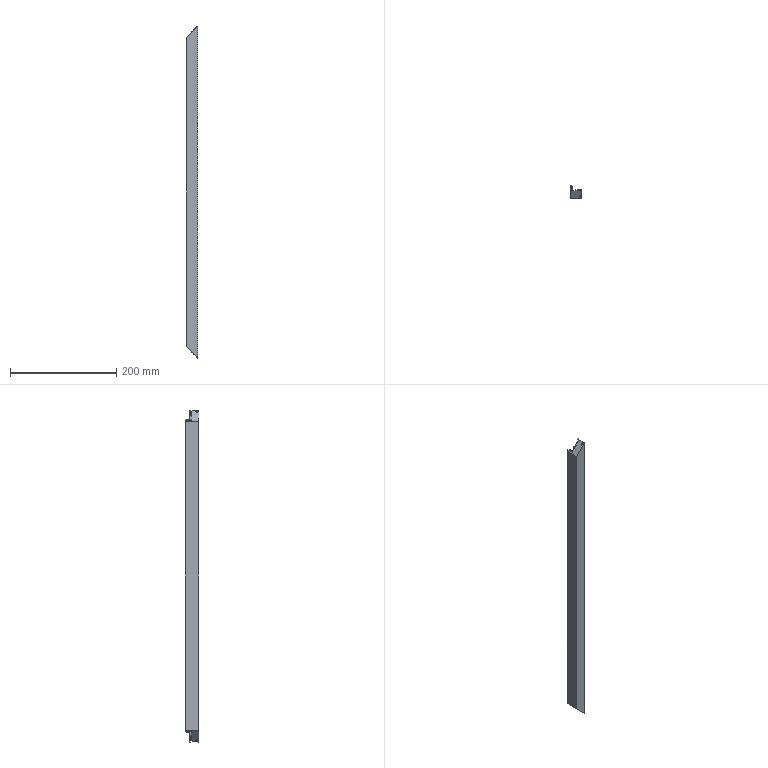Part | SolidWorks | features Extrusion 1, ICE 1 | 1 solid | 39 faces | box 22 x 25 x 624 mm | volume 198799 mm3 | plane 22 | cylinder 17 | commonest cylinder face diameters 0.6 x2 2 x2 3.8 x2 23.6 x2 26 x2 0.97 x1
STEP:
#1=CARTESIAN_POINT('',(27.064,65.097,604.634));
#2=VERTEX_POINT('',#1);
#3=CARTESIAN_POINT('',(26.938,66.899,604.509));
#4=VERTEX_POINT('',#3);
#5=CARTESIAN_POINT('',(27.064,65.097,604.634));
#6=CARTESIAN_POINT('',(26.98,65.694,604.55));
#7=CARTESIAN_POINT('',(26.938,66.296,604.509));
#8=CARTESIAN_POINT('',(26.938,66.899,604.509));
#9=(BOUNDED_CURVE()B_SPLINE_CURVE(3,(#5,#6,#7,#8),.UNSPECIFIED.,.F.,.F.)B_SPLINE_CURVE_WITH_KNOTS((4,4),(6.144,6.283),.UNSPECIFIED.)CURVE()GEOMETRIC_REPRESENTATION_ITEM()RATIONAL_B_SPLINE_CURVE((1.,0.9984,0.9984,1.))REPRESENTATION_ITEM(''));
#10=EDGE_CURVE('',#2,#4,#9,.T.);
#11=ORIENTED_EDGE('',*,*,#10,.T.);
#12=CARTESIAN_POINT('',(26.938,66.899,19.491));
#13=VERTEX_POINT('',#12);
#14=CARTESIAN_POINT('',(26.938,66.899,624.));
#15=DIRECTION('',(0.,0.,-1.));
#16=VECTOR('',#15,1000.);
#17=LINE('',#14,#16);
#18=EDGE_CURVE('',#4,#13,#17,.T.);
#19=ORIENTED_EDGE('',*,*,#18,.T.);
#20=CARTESIAN_POINT('',(27.064,65.097,19.366));
#21=VERTEX_POINT('',#20);
#22=CARTESIAN_POINT('',(26.938,66.899,19.491));
#23=CARTESIAN_POINT('',(26.938,66.296,19.491));
#24=CARTESIAN_POINT('',(26.98,65.694,19.45));
#25=CARTESIAN_POINT('',(27.064,65.097,19.366));
#26=(BOUNDED_CURVE()B_SPLINE_CURVE(3,(#22,#23,#24,#25),.UNSPECIFIED.,.F.,.F.)B_SPLINE_CURVE_WITH_KNOTS((4,4),(3.142,3.281),.UNSPECIFIED.)CURVE()GEOMETRIC_REPRESENTATION_ITEM()RATIONAL_B_SPLINE_CURVE((1.,0.9984,0.9984,1.))REPRESENTATION_ITEM(''));
#27=EDGE_CURVE('',#13,#21,#26,.T.);
#28=ORIENTED_EDGE('',*,*,#27,.T.);
#29=CARTESIAN_POINT('',(27.064,65.097,624.));
#30=DIRECTION('',(0.,0.,-1.));
#31=VECTOR('',#30,1000.);
#32=LINE('',#29,#31);
#33=EDGE_CURVE('',#2,#21,#32,.T.);
#34=ORIENTED_EDGE('',*,*,#33,.F.);
#35=EDGE_LOOP('',(#11,#19,#28,#34));
#36=FACE_OUTER_BOUND('',#35,.T.);
#37=CARTESIAN_POINT('',(39.938,66.899,624.));
#38=DIRECTION('',(0.,0.,-1.));
#39=DIRECTION('',(-1.,0.,0.));
#40=AXIS2_PLACEMENT_3D('',#37,#38,#39);
#41=CYLINDRICAL_SURFACE('',#40,13.);
#42=ADVANCED_FACE('',(#36),#41,.T.);
#43=CARTESIAN_POINT('',(28.252,68.536,605.823));
#44=VERTEX_POINT('',#43);
#45=CARTESIAN_POINT('',(28.138,66.899,605.709));
#46=VERTEX_POINT('',#45);
#47=CARTESIAN_POINT('',(28.252,68.536,605.823));
#48=CARTESIAN_POINT('',(28.176,67.993,605.747));
#49=CARTESIAN_POINT('',(28.138,67.447,605.709));
#50=CARTESIAN_POINT('',(28.138,66.899,605.709));
#51=(BOUNDED_CURVE()B_SPLINE_CURVE(3,(#47,#48,#49,#50),.UNSPECIFIED.,.F.,.F.)B_SPLINE_CURVE_WITH_KNOTS((4,4),(6.144,6.283),.UNSPECIFIED.)CURVE()GEOMETRIC_REPRESENTATION_ITEM()RATIONAL_B_SPLINE_CURVE((1.,0.9984,0.9984,1.))REPRESENTATION_ITEM(''));
#52=EDGE_CURVE('',#44,#46,#51,.T.);
#53=ORIENTED_EDGE('',*,*,#52,.T.);
#54=CARTESIAN_POINT('',(28.138,66.899,18.291));
#55=VERTEX_POINT('',#54);
#56=CARTESIAN_POINT('',(28.138,66.899,624.));
#57=DIRECTION('',(0.,0.,-1.));
#58=VECTOR('',#57,1000.);
#59=LINE('',#56,#58);
#60=EDGE_CURVE('',#46,#55,#59,.T.);
#61=ORIENTED_EDGE('',*,*,#60,.T.);
#62=CARTESIAN_POINT('',(28.252,68.536,18.177));
#63=VERTEX_POINT('',#62);
#64=CARTESIAN_POINT('',(28.138,66.899,18.291));
#65=CARTESIAN_POINT('',(28.138,67.447,18.291));
#66=CARTESIAN_POINT('',(28.176,67.993,18.253));
#67=CARTESIAN_POINT('',(28.252,68.536,18.177));
#68=(BOUNDED_CURVE()B_SPLINE_CURVE(3,(#64,#65,#66,#67),.UNSPECIFIED.,.F.,.F.)B_SPLINE_CURVE_WITH_KNOTS((4,4),(3.142,3.281),.UNSPECIFIED.)CURVE()GEOMETRIC_REPRESENTATION_ITEM()RATIONAL_B_SPLINE_CURVE((1.,0.9984,0.9984,1.))REPRESENTATION_ITEM(''));
#69=EDGE_CURVE('',#55,#63,#68,.T.);
#70=ORIENTED_EDGE('',*,*,#69,.T.);
#71=CARTESIAN_POINT('',(28.252,68.536,624.));
#72=DIRECTION('',(0.,0.,-1.));
#73=VECTOR('',#72,1000.);
#74=LINE('',#71,#73);
#75=EDGE_CURVE('',#44,#63,#74,.T.);
#76=ORIENTED_EDGE('',*,*,#75,.F.);
#77=EDGE_LOOP('',(#53,#61,#70,#76));
#78=FACE_OUTER_BOUND('',#77,.T.);
#79=CARTESIAN_POINT('',(39.938,66.899,624.));
#80=DIRECTION('',(0.,0.,-1.));
#81=DIRECTION('',(-1.,0.,0.));
#82=AXIS2_PLACEMENT_3D('',#79,#80,#81);
#83=CYLINDRICAL_SURFACE('',#82,11.8);
#84=ADVANCED_FACE('',(#78),#83,.F.);
#85=CARTESIAN_POINT('',(44.608,52.847,622.178));
#86=VERTEX_POINT('',#85);
#87=CARTESIAN_POINT('',(41.6,51.304,619.17));
#88=VERTEX_POINT('',#87);
#89=CARTESIAN_POINT('',(44.608,52.847,622.178));
#90=CARTESIAN_POINT('',(43.172,53.878,620.743));
#91=CARTESIAN_POINT('',(41.6,53.071,619.17));
#92=CARTESIAN_POINT('',(41.6,51.304,619.17));
#93=(BOUNDED_CURVE()B_SPLINE_CURVE(3,(#89,#90,#91,#92),.UNSPECIFIED.,.F.,.F.)B_SPLINE_CURVE_WITH_KNOTS((4,4),(4.09,6.283),.UNSPECIFIED.)CURVE()GEOMETRIC_REPRESENTATION_ITEM()RATIONAL_B_SPLINE_CURVE((1.,0.6376,0.6376,1.))REPRESENTATION_ITEM(''));
#94=EDGE_CURVE('',#86,#88,#93,.T.);
#95=ORIENTED_EDGE('',*,*,#94,.T.);
#96=CARTESIAN_POINT('',(41.6,51.304,4.83));
#97=VERTEX_POINT('',#96);
#98=CARTESIAN_POINT('',(41.6,51.304,624.));
#99=DIRECTION('',(0.,0.,-1.));
#100=VECTOR('',#99,1000.);
#101=LINE('',#98,#100);
#102=EDGE_CURVE('',#88,#97,#101,.T.);
#103=ORIENTED_EDGE('',*,*,#102,.T.);
#104=CARTESIAN_POINT('',(44.608,52.847,1.822));
#105=VERTEX_POINT('',#104);
#106=CARTESIAN_POINT('',(41.6,51.304,4.83));
#107=CARTESIAN_POINT('',(41.6,53.071,4.83));
#108=CARTESIAN_POINT('',(43.172,53.878,3.257));
#109=CARTESIAN_POINT('',(44.608,52.847,1.822));
#110=(BOUNDED_CURVE()B_SPLINE_CURVE(3,(#106,#107,#108,#109),.UNSPECIFIED.,.F.,.F.)B_SPLINE_CURVE_WITH_KNOTS((4,4),(3.142,5.335),.UNSPECIFIED.)CURVE()GEOMETRIC_REPRESENTATION_ITEM()RATIONAL_B_SPLINE_CURVE((1.,0.6376,0.6376,1.))REPRESENTATION_ITEM(''));
#111=EDGE_CURVE('',#97,#105,#110,.T.);
#112=ORIENTED_EDGE('',*,*,#111,.T.);
#113=CARTESIAN_POINT('',(44.608,52.847,624.));
#114=DIRECTION('',(0.,0.,-1.));
#115=VECTOR('',#114,1000.);
#116=LINE('',#113,#115);
#117=EDGE_CURVE('',#86,#105,#116,.T.);
#118=ORIENTED_EDGE('',*,*,#117,.F.);
#119=EDGE_LOOP('',(#95,#103,#112,#118));
#120=FACE_OUTER_BOUND('',#119,.T.);
#121=CARTESIAN_POINT('',(43.5,51.304,624.));
#122=DIRECTION('',(0.,0.,-1.));
#123=DIRECTION('',(-1.,0.,0.));
#124=AXIS2_PLACEMENT_3D('',#121,#122,#123);
#125=CYLINDRICAL_SURFACE('',#124,1.9);
#126=ADVANCED_FACE('',(#120),#125,.F.);
#127=CARTESIAN_POINT('',(45.44,49.348,623.01));
#128=VERTEX_POINT('',#127);
#129=CARTESIAN_POINT('',(45.43,49.204,623.));
#130=VERTEX_POINT('',#129);
#131=CARTESIAN_POINT('',(45.44,49.348,623.01));
#132=CARTESIAN_POINT('',(45.433,49.3,623.003));
#133=CARTESIAN_POINT('',(45.43,49.252,623.));
#134=CARTESIAN_POINT('',(45.43,49.204,623.));
#135=(BOUNDED_CURVE()B_SPLINE_CURVE(3,(#131,#132,#133,#134),.UNSPECIFIED.,.F.,.F.)B_SPLINE_CURVE_WITH_KNOTS((4,4),(6.138,6.283),.UNSPECIFIED.)CURVE()GEOMETRIC_REPRESENTATION_ITEM()RATIONAL_B_SPLINE_CURVE((1.,0.9983,0.9983,1.))REPRESENTATION_ITEM(''));
#136=EDGE_CURVE('',#128,#130,#135,.T.);
#137=ORIENTED_EDGE('',*,*,#136,.T.);
#138=CARTESIAN_POINT('',(45.43,49.204,1.));
#139=VERTEX_POINT('',#138);
#140=CARTESIAN_POINT('',(45.43,49.204,624.));
#141=DIRECTION('',(0.,0.,-1.));
#142=VECTOR('',#141,1000.);
#143=LINE('',#140,#142);
#144=EDGE_CURVE('',#130,#139,#143,.T.);
#145=ORIENTED_EDGE('',*,*,#144,.T.);
#146=CARTESIAN_POINT('',(45.44,49.348,0.9896));
#147=VERTEX_POINT('',#146);
#148=CARTESIAN_POINT('',(45.43,49.204,1.));
#149=CARTESIAN_POINT('',(45.43,49.252,1.));
#150=CARTESIAN_POINT('',(45.433,49.3,0.9965));
#151=CARTESIAN_POINT('',(45.44,49.348,0.9896));
#152=(BOUNDED_CURVE()B_SPLINE_CURVE(3,(#148,#149,#150,#151),.UNSPECIFIED.,.F.,.F.)B_SPLINE_CURVE_WITH_KNOTS((4,4),(3.142,3.286),.UNSPECIFIED.)CURVE()GEOMETRIC_REPRESENTATION_ITEM()RATIONAL_B_SPLINE_CURVE((1.,0.9983,0.9983,1.))REPRESENTATION_ITEM(''));
#153=EDGE_CURVE('',#139,#147,#152,.T.);
#154=ORIENTED_EDGE('',*,*,#153,.T.);
#155=CARTESIAN_POINT('',(45.44,49.348,624.));
#156=DIRECTION('',(0.,0.,-1.));
#157=VECTOR('',#156,1000.);
#158=LINE('',#155,#157);
#159=EDGE_CURVE('',#128,#147,#158,.T.);
#160=ORIENTED_EDGE('',*,*,#159,.F.);
#161=EDGE_LOOP('',(#137,#145,#154,#160));
#162=FACE_OUTER_BOUND('',#161,.T.);
#163=CARTESIAN_POINT('',(46.43,49.204,624.));
#164=DIRECTION('',(0.,0.,-1.));
#165=DIRECTION('',(-1.,0.,0.));
#166=AXIS2_PLACEMENT_3D('',#163,#164,#165);
#167=CYLINDRICAL_SURFACE('',#166,1.);
#168=ADVANCED_FACE('',(#162),#167,.F.);
#169=CARTESIAN_POINT('',(24.43,73.204,602.));
#170=VERTEX_POINT('',#169);
#171=CARTESIAN_POINT('',(24.43,73.204,22.));
#172=VERTEX_POINT('',#171);
#173=CARTESIAN_POINT('',(24.43,73.204,624.));
#174=DIRECTION('',(0.,0.,-1.));
#175=VECTOR('',#174,1000.);
#176=LINE('',#173,#175);
#177=EDGE_CURVE('',#170,#172,#176,.T.);
#178=ORIENTED_EDGE('',*,*,#177,.T.);
#179=CARTESIAN_POINT('',(24.43,48.204,22.));
#180=VERTEX_POINT('',#179);
#181=CARTESIAN_POINT('',(24.43,78.204,22.));
#182=DIRECTION('',(0.,-1.,0.));
#183=VECTOR('',#182,1000.);
#184=LINE('',#181,#183);
#185=EDGE_CURVE('',#172,#180,#184,.T.);
#186=ORIENTED_EDGE('',*,*,#185,.T.);
#187=CARTESIAN_POINT('',(24.43,48.204,602.));
#188=VERTEX_POINT('',#187);
#189=CARTESIAN_POINT('',(24.43,48.204,624.));
#190=DIRECTION('',(0.,0.,-1.));
#191=VECTOR('',#190,1000.);
#192=LINE('',#189,#191);
#193=EDGE_CURVE('',#188,#180,#192,.T.);
#194=ORIENTED_EDGE('',*,*,#193,.F.);
#195=CARTESIAN_POINT('',(24.43,78.204,602.));
#196=DIRECTION('',(0.,-1.,0.));
#197=VECTOR('',#196,1000.);
#198=LINE('',#195,#197);
#199=EDGE_CURVE('',#170,#188,#198,.T.);
#200=ORIENTED_EDGE('',*,*,#199,.F.);
#201=EDGE_LOOP('',(#178,#186,#194,#200));
#202=FACE_OUTER_BOUND('',#201,.T.);
#203=CARTESIAN_POINT('',(24.43,48.204,624.));
#204=DIRECTION('',(1.,0.,0.));
#205=DIRECTION('',(0.,0.,-1.));
#206=AXIS2_PLACEMENT_3D('',#203,#204,#205);
#207=PLANE('',#206);
#208=ADVANCED_FACE('',(#202),#207,.F.);
#209=ORIENTED_EDGE('',*,*,#193,.T.);
#210=CARTESIAN_POINT('',(46.43,48.204,0.));
#211=VERTEX_POINT('',#210);
#212=CARTESIAN_POINT('',(24.43,48.204,22.));
#213=DIRECTION('',(-0.7071,0.,0.7071));
#214=VECTOR('',#213,1000.);
#215=LINE('',#212,#214);
#216=EDGE_CURVE('',#211,#180,#215,.T.);
#217=ORIENTED_EDGE('',*,*,#216,.F.);
#218=CARTESIAN_POINT('',(46.43,48.204,624.));
#219=VERTEX_POINT('',#218);
#220=CARTESIAN_POINT('',(46.43,48.204,624.));
#221=DIRECTION('',(0.,0.,-1.));
#222=VECTOR('',#221,1000.);
#223=LINE('',#220,#222);
#224=EDGE_CURVE('',#219,#211,#223,.T.);
#225=ORIENTED_EDGE('',*,*,#224,.F.);
#226=CARTESIAN_POINT('',(24.43,48.204,602.));
#227=DIRECTION('',(0.7071,0.,0.7071));
#228=VECTOR('',#227,1000.);
#229=LINE('',#226,#228);
#230=EDGE_CURVE('',#188,#219,#229,.T.);
#231=ORIENTED_EDGE('',*,*,#230,.F.);
#232=EDGE_LOOP('',(#209,#217,#225,#231));
#233=FACE_OUTER_BOUND('',#232,.T.);
#234=CARTESIAN_POINT('',(24.43,48.204,624.));
#235=DIRECTION('',(0.,1.,0.));
#236=DIRECTION('',(0.,0.,1.));
#237=AXIS2_PLACEMENT_3D('',#234,#235,#236);
#238=PLANE('',#237);
#239=ADVANCED_FACE('',(#233),#238,.F.);
#240=ORIENTED_EDGE('',*,*,#144,.F.);
#241=CARTESIAN_POINT('',(45.43,49.204,623.));
#242=CARTESIAN_POINT('',(45.43,48.618,623.));
#243=CARTESIAN_POINT('',(45.844,48.204,623.414));
#244=CARTESIAN_POINT('',(46.43,48.204,624.));
#245=(BOUNDED_CURVE()B_SPLINE_CURVE(3,(#241,#242,#243,#244),.UNSPECIFIED.,.F.,.F.)B_SPLINE_CURVE_WITH_KNOTS((4,4),(0.,1.571),.UNSPECIFIED.)CURVE()GEOMETRIC_REPRESENTATION_ITEM()RATIONAL_B_SPLINE_CURVE((1.,0.8047,0.8047,1.))REPRESENTATION_ITEM(''));
#246=EDGE_CURVE('',#130,#219,#245,.T.);
#247=ORIENTED_EDGE('',*,*,#246,.T.);
#248=ORIENTED_EDGE('',*,*,#224,.T.);
#249=CARTESIAN_POINT('',(46.43,48.204,0.));
#250=CARTESIAN_POINT('',(45.844,48.204,0.5858));
#251=CARTESIAN_POINT('',(45.43,48.618,1.));
#252=CARTESIAN_POINT('',(45.43,49.204,1.));
#253=(BOUNDED_CURVE()B_SPLINE_CURVE(3,(#249,#250,#251,#252),.UNSPECIFIED.,.F.,.F.)B_SPLINE_CURVE_WITH_KNOTS((4,4),(1.571,3.142),.UNSPECIFIED.)CURVE()GEOMETRIC_REPRESENTATION_ITEM()RATIONAL_B_SPLINE_CURVE((1.,0.8047,0.8047,1.))REPRESENTATION_ITEM(''));
#254=EDGE_CURVE('',#211,#139,#253,.T.);
#255=ORIENTED_EDGE('',*,*,#254,.T.);
#256=EDGE_LOOP('',(#240,#247,#248,#255));
#257=FACE_OUTER_BOUND('',#256,.T.);
#258=CARTESIAN_POINT('',(46.43,49.204,624.));
#259=DIRECTION('',(0.,0.,-1.));
#260=DIRECTION('',(-1.,0.,0.));
#261=AXIS2_PLACEMENT_3D('',#258,#259,#260);
#262=CYLINDRICAL_SURFACE('',#261,1.);
#263=ADVANCED_FACE('',(#257),#262,.F.);
#264=ORIENTED_EDGE('',*,*,#159,.T.);
#265=CARTESIAN_POINT('',(44.663,49.801,1.767));
#266=VERTEX_POINT('',#265);
#267=CARTESIAN_POINT('',(45.44,49.348,0.9896));
#268=CARTESIAN_POINT('',(45.514,49.857,0.9153));
#269=CARTESIAN_POINT('',(45.07,50.116,1.36));
#270=CARTESIAN_POINT('',(44.663,49.801,1.767));
#271=(BOUNDED_CURVE()B_SPLINE_CURVE(3,(#267,#268,#269,#270),.UNSPECIFIED.,.F.,.F.)B_SPLINE_CURVE_WITH_KNOTS((4,4),(6.138,8.513),.UNSPECIFIED.)CURVE()GEOMETRIC_REPRESENTATION_ITEM()RATIONAL_B_SPLINE_CURVE((1.,0.5828,0.5828,1.))REPRESENTATION_ITEM(''));
#272=EDGE_CURVE('',#147,#266,#271,.T.);
#273=ORIENTED_EDGE('',*,*,#272,.T.);
#274=CARTESIAN_POINT('',(44.663,49.801,622.233));
#275=VERTEX_POINT('',#274);
#276=CARTESIAN_POINT('',(44.663,49.801,624.));
#277=DIRECTION('',(0.,0.,-1.));
#278=VECTOR('',#277,1000.);
#279=LINE('',#276,#278);
#280=EDGE_CURVE('',#275,#266,#279,.T.);
#281=ORIENTED_EDGE('',*,*,#280,.F.);
#282=CARTESIAN_POINT('',(44.663,49.801,622.233));
#283=CARTESIAN_POINT('',(45.07,50.116,622.64));
#284=CARTESIAN_POINT('',(45.514,49.857,623.085));
#285=CARTESIAN_POINT('',(45.44,49.348,623.01));
#286=(BOUNDED_CURVE()B_SPLINE_CURVE(3,(#282,#283,#284,#285),.UNSPECIFIED.,.F.,.F.)B_SPLINE_CURVE_WITH_KNOTS((4,4),(0.9119,3.286),.UNSPECIFIED.)CURVE()GEOMETRIC_REPRESENTATION_ITEM()RATIONAL_B_SPLINE_CURVE((1.,0.5828,0.5828,1.))REPRESENTATION_ITEM(''));
#287=EDGE_CURVE('',#275,#128,#286,.T.);
#288=ORIENTED_EDGE('',*,*,#287,.T.);
#289=EDGE_LOOP('',(#264,#273,#281,#288));
#290=FACE_OUTER_BOUND('',#289,.T.);
#291=CARTESIAN_POINT('',(44.96,49.418,624.));
#292=DIRECTION('',(0.,0.,-1.));
#293=DIRECTION('',(-1.,0.,0.));
#294=AXIS2_PLACEMENT_3D('',#291,#292,#293);
#295=CYLINDRICAL_SURFACE('',#294,0.4852);
#296=ADVANCED_FACE('',(#290),#295,.T.);
#297=ORIENTED_EDGE('',*,*,#102,.F.);
#298=CARTESIAN_POINT('',(41.6,51.304,619.17));
#299=CARTESIAN_POINT('',(41.6,49.489,619.17));
#300=CARTESIAN_POINT('',(43.228,48.691,620.799));
#301=CARTESIAN_POINT('',(44.663,49.801,622.233));
#302=(BOUNDED_CURVE()B_SPLINE_CURVE(3,(#298,#299,#300,#301),.UNSPECIFIED.,.F.,.F.)B_SPLINE_CURVE_WITH_KNOTS((4,4),(0.,2.23),.UNSPECIFIED.)CURVE()GEOMETRIC_REPRESENTATION_ITEM()RATIONAL_B_SPLINE_CURVE((1.,0.6269,0.6269,1.))REPRESENTATION_ITEM(''));
#303=EDGE_CURVE('',#88,#275,#302,.T.);
#304=ORIENTED_EDGE('',*,*,#303,.T.);
#305=ORIENTED_EDGE('',*,*,#280,.T.);
#306=CARTESIAN_POINT('',(44.663,49.801,1.767));
#307=CARTESIAN_POINT('',(43.228,48.691,3.201));
#308=CARTESIAN_POINT('',(41.6,49.489,4.83));
#309=CARTESIAN_POINT('',(41.6,51.304,4.83));
#310=(BOUNDED_CURVE()B_SPLINE_CURVE(3,(#306,#307,#308,#309),.UNSPECIFIED.,.F.,.F.)B_SPLINE_CURVE_WITH_KNOTS((4,4),(0.9119,3.142),.UNSPECIFIED.)CURVE()GEOMETRIC_REPRESENTATION_ITEM()RATIONAL_B_SPLINE_CURVE((1.,0.6269,0.6269,1.))REPRESENTATION_ITEM(''));
#311=EDGE_CURVE('',#266,#97,#310,.T.);
#312=ORIENTED_EDGE('',*,*,#311,.T.);
#313=EDGE_LOOP('',(#297,#304,#305,#312));
#314=FACE_OUTER_BOUND('',#313,.T.);
#315=CARTESIAN_POINT('',(43.5,51.304,624.));
#316=DIRECTION('',(0.,0.,-1.));
#317=DIRECTION('',(-1.,0.,0.));
#318=AXIS2_PLACEMENT_3D('',#315,#316,#317);
#319=CYLINDRICAL_SURFACE('',#318,1.9);
#320=ADVANCED_FACE('',(#314),#319,.F.);
#321=ORIENTED_EDGE('',*,*,#117,.T.);
#322=CARTESIAN_POINT('',(45.4,53.253,1.03));
#323=VERTEX_POINT('',#322);
#324=CARTESIAN_POINT('',(44.608,52.847,1.822));
#325=CARTESIAN_POINT('',(44.986,52.575,1.444));
#326=CARTESIAN_POINT('',(45.4,52.788,1.03));
#327=CARTESIAN_POINT('',(45.4,53.253,1.03));
#328=(BOUNDED_CURVE()B_SPLINE_CURVE(3,(#324,#325,#326,#327),.UNSPECIFIED.,.F.,.F.)B_SPLINE_CURVE_WITH_KNOTS((4,4),(4.09,6.283),.UNSPECIFIED.)CURVE()GEOMETRIC_REPRESENTATION_ITEM()RATIONAL_B_SPLINE_CURVE((1.,0.6376,0.6376,1.))REPRESENTATION_ITEM(''));
#329=EDGE_CURVE('',#105,#323,#328,.T.);
#330=ORIENTED_EDGE('',*,*,#329,.T.);
#331=CARTESIAN_POINT('',(45.4,53.253,622.97));
#332=VERTEX_POINT('',#331);
#333=CARTESIAN_POINT('',(45.4,53.253,624.));
#334=DIRECTION('',(0.,0.,-1.));
#335=VECTOR('',#334,1000.);
#336=LINE('',#333,#335);
#337=EDGE_CURVE('',#332,#323,#336,.T.);
#338=ORIENTED_EDGE('',*,*,#337,.F.);
#339=CARTESIAN_POINT('',(45.4,53.253,622.97));
#340=CARTESIAN_POINT('',(45.4,52.788,622.97));
#341=CARTESIAN_POINT('',(44.986,52.575,622.556));
#342=CARTESIAN_POINT('',(44.608,52.847,622.178));
#343=(BOUNDED_CURVE()B_SPLINE_CURVE(3,(#339,#340,#341,#342),.UNSPECIFIED.,.F.,.F.)B_SPLINE_CURVE_WITH_KNOTS((4,4),(3.142,5.335),.UNSPECIFIED.)CURVE()GEOMETRIC_REPRESENTATION_ITEM()RATIONAL_B_SPLINE_CURVE((1.,0.6376,0.6376,1.))REPRESENTATION_ITEM(''));
#344=EDGE_CURVE('',#332,#86,#343,.T.);
#345=ORIENTED_EDGE('',*,*,#344,.T.);
#346=EDGE_LOOP('',(#321,#330,#338,#345));
#347=FACE_OUTER_BOUND('',#346,.T.);
#348=CARTESIAN_POINT('',(44.9,53.253,624.));
#349=DIRECTION('',(0.,0.,-1.));
#350=DIRECTION('',(-1.,0.,0.));
#351=AXIS2_PLACEMENT_3D('',#348,#349,#350);
#352=CYLINDRICAL_SURFACE('',#351,0.5);
#353=ADVANCED_FACE('',(#347),#352,.T.);
#354=ORIENTED_EDGE('',*,*,#337,.T.);
#355=CARTESIAN_POINT('',(45.4,58.567,1.03));
#356=VERTEX_POINT('',#355);
#357=CARTESIAN_POINT('',(45.4,58.567,1.03));
#358=DIRECTION('',(0.,1.,0.));
#359=VECTOR('',#358,1000.);
#360=LINE('',#357,#359);
#361=EDGE_CURVE('',#323,#356,#360,.T.);
#362=ORIENTED_EDGE('',*,*,#361,.T.);
#363=CARTESIAN_POINT('',(45.4,58.567,622.97));
#364=VERTEX_POINT('',#363);
#365=CARTESIAN_POINT('',(45.4,58.567,624.));
#366=DIRECTION('',(0.,0.,-1.));
#367=VECTOR('',#366,1000.);
#368=LINE('',#365,#367);
#369=EDGE_CURVE('',#364,#356,#368,.T.);
#370=ORIENTED_EDGE('',*,*,#369,.F.);
#371=CARTESIAN_POINT('',(45.4,58.567,622.97));
#372=DIRECTION('',(0.,-1.,0.));
#373=VECTOR('',#372,1000.);
#374=LINE('',#371,#373);
#375=EDGE_CURVE('',#364,#332,#374,.T.);
#376=ORIENTED_EDGE('',*,*,#375,.T.);
#377=EDGE_LOOP('',(#354,#362,#370,#376));
#378=FACE_OUTER_BOUND('',#377,.T.);
#379=CARTESIAN_POINT('',(45.4,58.567,624.));
#380=DIRECTION('',(-1.,0.,0.));
#381=DIRECTION('',(0.,0.,1.));
#382=AXIS2_PLACEMENT_3D('',#379,#380,#381);
#383=PLANE('',#382);
#384=ADVANCED_FACE('',(#378),#383,.F.);
#385=ORIENTED_EDGE('',*,*,#369,.T.);
#386=CARTESIAN_POINT('',(41.4,62.567,5.03));
#387=VERTEX_POINT('',#386);
#388=CARTESIAN_POINT('',(45.4,58.567,1.03));
#389=CARTESIAN_POINT('',(45.4,60.91,1.03));
#390=CARTESIAN_POINT('',(43.743,62.567,2.687));
#391=CARTESIAN_POINT('',(41.4,62.567,5.03));
#392=(BOUNDED_CURVE()B_SPLINE_CURVE(3,(#388,#389,#390,#391),.UNSPECIFIED.,.F.,.F.)B_SPLINE_CURVE_WITH_KNOTS((4,4),(0.,1.571),.UNSPECIFIED.)CURVE()GEOMETRIC_REPRESENTATION_ITEM()RATIONAL_B_SPLINE_CURVE((1.,0.8047,0.8047,1.))REPRESENTATION_ITEM(''));
#393=EDGE_CURVE('',#356,#387,#392,.T.);
#394=ORIENTED_EDGE('',*,*,#393,.T.);
#395=CARTESIAN_POINT('',(41.4,62.567,618.97));
#396=VERTEX_POINT('',#395);
#397=CARTESIAN_POINT('',(41.4,62.567,624.));
#398=DIRECTION('',(0.,0.,-1.));
#399=VECTOR('',#398,1000.);
#400=LINE('',#397,#399);
#401=EDGE_CURVE('',#396,#387,#400,.T.);
#402=ORIENTED_EDGE('',*,*,#401,.F.);
#403=CARTESIAN_POINT('',(41.4,62.567,618.97));
#404=CARTESIAN_POINT('',(43.743,62.567,621.313));
#405=CARTESIAN_POINT('',(45.4,60.91,622.97));
#406=CARTESIAN_POINT('',(45.4,58.567,622.97));
#407=(BOUNDED_CURVE()B_SPLINE_CURVE(3,(#403,#404,#405,#406),.UNSPECIFIED.,.F.,.F.)B_SPLINE_CURVE_WITH_KNOTS((4,4),(1.571,3.142),.UNSPECIFIED.)CURVE()GEOMETRIC_REPRESENTATION_ITEM()RATIONAL_B_SPLINE_CURVE((1.,0.8047,0.8047,1.))REPRESENTATION_ITEM(''));
#408=EDGE_CURVE('',#396,#364,#407,.T.);
#409=ORIENTED_EDGE('',*,*,#408,.T.);
#410=EDGE_LOOP('',(#385,#394,#402,#409));
#411=FACE_OUTER_BOUND('',#410,.T.);
#412=CARTESIAN_POINT('',(41.4,58.567,624.));
#413=DIRECTION('',(0.,0.,-1.));
#414=DIRECTION('',(-1.,0.,0.));
#415=AXIS2_PLACEMENT_3D('',#412,#413,#414);
#416=CYLINDRICAL_SURFACE('',#415,4.);
#417=ADVANCED_FACE('',(#411),#416,.T.);
#418=ORIENTED_EDGE('',*,*,#401,.T.);
#419=CARTESIAN_POINT('',(35.32,62.567,11.11));
#420=VERTEX_POINT('',#419);
#421=CARTESIAN_POINT('',(-271.125,62.567,317.555));
#422=DIRECTION('',(-0.7071,0.,0.7071));
#423=VECTOR('',#422,1000.);
#424=LINE('',#421,#423);
#425=EDGE_CURVE('',#387,#420,#424,.T.);
#426=ORIENTED_EDGE('',*,*,#425,.T.);
#427=CARTESIAN_POINT('',(35.32,62.567,612.89));
#428=VERTEX_POINT('',#427);
#429=CARTESIAN_POINT('',(35.32,62.567,624.));
#430=DIRECTION('',(0.,0.,-1.));
#431=VECTOR('',#430,1000.);
#432=LINE('',#429,#431);
#433=EDGE_CURVE('',#428,#420,#432,.T.);
#434=ORIENTED_EDGE('',*,*,#433,.F.);
#435=CARTESIAN_POINT('',(40.875,62.567,618.445));
#436=DIRECTION('',(0.7071,0.,0.7071));
#437=VECTOR('',#436,1000.);
#438=LINE('',#435,#437);
#439=EDGE_CURVE('',#428,#396,#438,.T.);
#440=ORIENTED_EDGE('',*,*,#439,.T.);
#441=EDGE_LOOP('',(#418,#426,#434,#440));
#442=FACE_OUTER_BOUND('',#441,.T.);
#443=CARTESIAN_POINT('',(35.32,62.567,624.));
#444=DIRECTION('',(0.,-1.,0.));
#445=DIRECTION('',(0.,0.,-1.));
#446=AXIS2_PLACEMENT_3D('',#443,#444,#445);
#447=PLANE('',#446);
#448=ADVANCED_FACE('',(#442),#447,.F.);
#449=ORIENTED_EDGE('',*,*,#433,.T.);
#450=CARTESIAN_POINT('',(35.32,63.565,11.11));
#451=VERTEX_POINT('',#450);
#452=CARTESIAN_POINT('',(35.32,63.565,11.11));
#453=DIRECTION('',(0.,1.,0.));
#454=VECTOR('',#453,1000.);
#455=LINE('',#452,#454);
#456=EDGE_CURVE('',#420,#451,#455,.T.);
#457=ORIENTED_EDGE('',*,*,#456,.T.);
#458=CARTESIAN_POINT('',(35.32,63.565,612.89));
#459=VERTEX_POINT('',#458);
#460=CARTESIAN_POINT('',(35.32,63.565,624.));
#461=DIRECTION('',(0.,0.,-1.));
#462=VECTOR('',#461,1000.);
#463=LINE('',#460,#462);
#464=EDGE_CURVE('',#459,#451,#463,.T.);
#465=ORIENTED_EDGE('',*,*,#464,.F.);
#466=CARTESIAN_POINT('',(35.32,63.565,612.89));
#467=DIRECTION('',(0.,-1.,0.));
#468=VECTOR('',#467,1000.);
#469=LINE('',#466,#468);
#470=EDGE_CURVE('',#459,#428,#469,.T.);
#471=ORIENTED_EDGE('',*,*,#470,.T.);
#472=EDGE_LOOP('',(#449,#457,#465,#471));
#473=FACE_OUTER_BOUND('',#472,.T.);
#474=CARTESIAN_POINT('',(35.32,63.565,624.));
#475=DIRECTION('',(-1.,0.,0.));
#476=DIRECTION('',(0.,0.,1.));
#477=AXIS2_PLACEMENT_3D('',#474,#475,#476);
#478=PLANE('',#477);
#479=ADVANCED_FACE('',(#473),#478,.F.);
#480=ORIENTED_EDGE('',*,*,#464,.T.);
#481=CARTESIAN_POINT('',(37.522,63.233,8.907));
#482=VERTEX_POINT('',#481);
#483=CARTESIAN_POINT('',(35.32,63.565,11.11));
#484=CARTESIAN_POINT('',(36.066,63.548,10.364));
#485=CARTESIAN_POINT('',(36.804,63.437,9.625));
#486=CARTESIAN_POINT('',(37.522,63.233,8.907));
#487=(BOUNDED_CURVE()B_SPLINE_CURVE(3,(#483,#484,#485,#486),.UNSPECIFIED.,.F.,.F.)B_SPLINE_CURVE_WITH_KNOTS((4,4),(4.735,4.989),.UNSPECIFIED.)CURVE()GEOMETRIC_REPRESENTATION_ITEM()RATIONAL_B_SPLINE_CURVE((1.,0.9946,0.9946,1.))REPRESENTATION_ITEM(''));
#488=EDGE_CURVE('',#451,#482,#487,.T.);
#489=ORIENTED_EDGE('',*,*,#488,.T.);
#490=CARTESIAN_POINT('',(37.522,63.233,615.093));
#491=VERTEX_POINT('',#490);
#492=CARTESIAN_POINT('',(37.522,63.233,624.));
#493=DIRECTION('',(0.,0.,-1.));
#494=VECTOR('',#493,1000.);
#495=LINE('',#492,#494);
#496=EDGE_CURVE('',#491,#482,#495,.T.);
#497=ORIENTED_EDGE('',*,*,#496,.F.);
#498=CARTESIAN_POINT('',(37.522,63.233,615.093));
#499=CARTESIAN_POINT('',(36.804,63.437,614.375));
#500=CARTESIAN_POINT('',(36.066,63.548,613.636));
#501=CARTESIAN_POINT('',(35.32,63.565,612.89));
#502=(BOUNDED_CURVE()B_SPLINE_CURVE(3,(#498,#499,#500,#501),.UNSPECIFIED.,.F.,.F.)B_SPLINE_CURVE_WITH_KNOTS((4,4),(4.436,4.69),.UNSPECIFIED.)CURVE()GEOMETRIC_REPRESENTATION_ITEM()RATIONAL_B_SPLINE_CURVE((1.,0.9946,0.9946,1.))REPRESENTATION_ITEM(''));
#503=EDGE_CURVE('',#491,#459,#502,.T.);
#504=ORIENTED_EDGE('',*,*,#503,.T.);
#505=EDGE_LOOP('',(#480,#489,#497,#504));
#506=FACE_OUTER_BOUND('',#505,.T.);
#507=CARTESIAN_POINT('',(35.12,54.767,624.));
#508=DIRECTION('',(0.,0.,-1.));
#509=DIRECTION('',(-1.,0.,0.));
#510=AXIS2_PLACEMENT_3D('',#507,#508,#509);
#511=CYLINDRICAL_SURFACE('',#510,8.8);
#512=ADVANCED_FACE('',(#506),#511,.F.);
#513=ORIENTED_EDGE('',*,*,#496,.T.);
#514=CARTESIAN_POINT('',(43.408,63.335,3.022));
#515=VERTEX_POINT('',#514);
#516=CARTESIAN_POINT('',(37.522,63.233,8.907));
#517=CARTESIAN_POINT('',(39.466,62.681,6.964));
#518=CARTESIAN_POINT('',(41.485,62.716,4.944));
#519=CARTESIAN_POINT('',(43.408,63.335,3.022));
#520=(BOUNDED_CURVE()B_SPLINE_CURVE(3,(#516,#517,#518,#519),.UNSPECIFIED.,.F.,.F.)B_SPLINE_CURVE_WITH_KNOTS((4,4),(4.436,5.024),.UNSPECIFIED.)CURVE()GEOMETRIC_REPRESENTATION_ITEM()RATIONAL_B_SPLINE_CURVE((1.,0.9714,0.9714,1.))REPRESENTATION_ITEM(''));
#521=EDGE_CURVE('',#482,#515,#520,.T.);
#522=ORIENTED_EDGE('',*,*,#521,.T.);
#523=CARTESIAN_POINT('',(43.408,63.335,620.978));
#524=VERTEX_POINT('',#523);
#525=CARTESIAN_POINT('',(43.408,63.335,624.));
#526=DIRECTION('',(0.,0.,-1.));
#527=VECTOR('',#526,1000.);
#528=LINE('',#525,#527);
#529=EDGE_CURVE('',#524,#515,#528,.T.);
#530=ORIENTED_EDGE('',*,*,#529,.F.);
#531=CARTESIAN_POINT('',(43.408,63.335,620.978));
#532=CARTESIAN_POINT('',(41.485,62.716,619.056));
#533=CARTESIAN_POINT('',(39.466,62.681,617.036));
#534=CARTESIAN_POINT('',(37.522,63.233,615.093));
#535=(BOUNDED_CURVE()B_SPLINE_CURVE(3,(#531,#532,#533,#534),.UNSPECIFIED.,.F.,.F.)B_SPLINE_CURVE_WITH_KNOTS((4,4),(4.401,4.989),.UNSPECIFIED.)CURVE()GEOMETRIC_REPRESENTATION_ITEM()RATIONAL_B_SPLINE_CURVE((1.,0.9714,0.9714,1.))REPRESENTATION_ITEM(''));
#536=EDGE_CURVE('',#524,#491,#535,.T.);
#537=ORIENTED_EDGE('',*,*,#536,.T.);
#538=EDGE_LOOP('',(#513,#522,#530,#537));
#539=FACE_OUTER_BOUND('',#538,.T.);
#540=CARTESIAN_POINT('',(40.297,73.007,624.));
#541=DIRECTION('',(0.,0.,-1.));
#542=DIRECTION('',(-1.,0.,0.));
#543=AXIS2_PLACEMENT_3D('',#540,#541,#542);
#544=CYLINDRICAL_SURFACE('',#543,10.16);
#545=ADVANCED_FACE('',(#539),#544,.T.);
#546=ORIENTED_EDGE('',*,*,#529,.T.);
#547=CARTESIAN_POINT('',(46.43,64.307,0.));
#548=VERTEX_POINT('',#547);
#549=CARTESIAN_POINT('',(-251.806,-31.633,298.236));
#550=DIRECTION('',(0.6895,0.2218,-0.6895));
#551=VECTOR('',#550,1000.);
#552=LINE('',#549,#551);
#553=EDGE_CURVE('',#515,#548,#552,.T.);
#554=ORIENTED_EDGE('',*,*,#553,.T.);
#555=CARTESIAN_POINT('',(46.43,64.307,624.));
#556=VERTEX_POINT('',#555);
#557=CARTESIAN_POINT('',(46.43,64.307,624.));
#558=DIRECTION('',(0.,0.,-1.));
#559=VECTOR('',#558,1000.);
#560=LINE('',#557,#559);
#561=EDGE_CURVE('',#556,#548,#560,.T.);
#562=ORIENTED_EDGE('',*,*,#561,.F.);
#563=CARTESIAN_POINT('',(44.844,63.797,622.415));
#564=DIRECTION('',(-0.6895,-0.2218,-0.6895));
#565=VECTOR('',#564,1000.);
#566=LINE('',#563,#565);
#567=EDGE_CURVE('',#556,#524,#566,.T.);
#568=ORIENTED_EDGE('',*,*,#567,.T.);
#569=EDGE_LOOP('',(#546,#554,#562,#568));
#570=FACE_OUTER_BOUND('',#569,.T.);
#571=CARTESIAN_POINT('',(43.408,63.335,624.));
#572=DIRECTION('',(-0.3062,0.952,0.));
#573=DIRECTION('',(-0.952,-0.3062,0.));
#574=AXIS2_PLACEMENT_3D('',#571,#572,#573);
#575=PLANE('',#574);
#576=ADVANCED_FACE('',(#570),#575,.F.);
#577=CARTESIAN_POINT('',(46.43,65.567,0.));
#578=VERTEX_POINT('',#577);
#579=CARTESIAN_POINT('',(46.43,65.567,0.));
#580=DIRECTION('',(0.,1.,0.));
#581=VECTOR('',#580,1000.);
#582=LINE('',#579,#581);
#583=EDGE_CURVE('',#548,#578,#582,.T.);
#584=ORIENTED_EDGE('',*,*,#583,.T.);
#585=CARTESIAN_POINT('',(46.43,65.567,624.));
#586=VERTEX_POINT('',#585);
#587=CARTESIAN_POINT('',(46.43,65.567,624.));
#588=DIRECTION('',(0.,0.,-1.));
#589=VECTOR('',#588,1000.);
#590=LINE('',#587,#589);
#591=EDGE_CURVE('',#586,#578,#590,.T.);
#592=ORIENTED_EDGE('',*,*,#591,.F.);
#593=CARTESIAN_POINT('',(46.43,65.567,624.));
#594=DIRECTION('',(0.,1.,0.));
#595=VECTOR('',#594,1000.);
#596=LINE('',#593,#595);
#597=EDGE_CURVE('',#556,#586,#596,.T.);
#598=ORIENTED_EDGE('',*,*,#597,.F.);
#599=ORIENTED_EDGE('',*,*,#561,.T.);
#600=EDGE_LOOP('',(#584,#592,#598,#599));
#601=FACE_OUTER_BOUND('',#600,.T.);
#602=CARTESIAN_POINT('',(46.43,65.567,624.));
#603=DIRECTION('',(-1.,0.,0.));
#604=DIRECTION('',(0.,0.,1.));
#605=AXIS2_PLACEMENT_3D('',#602,#603,#604);
#606=PLANE('',#605);
#607=ADVANCED_FACE('',(#601),#606,.F.);
#608=ORIENTED_EDGE('',*,*,#591,.T.);
#609=CARTESIAN_POINT('',(43.041,64.477,3.389));
#610=VERTEX_POINT('',#609);
#611=CARTESIAN_POINT('',(-251.999,-30.435,298.428));
#612=DIRECTION('',(-0.6895,-0.2218,0.6895));
#613=VECTOR('',#612,1000.);
#614=LINE('',#611,#613);
#615=EDGE_CURVE('',#578,#610,#614,.T.);
#616=ORIENTED_EDGE('',*,*,#615,.T.);
#617=CARTESIAN_POINT('',(43.041,64.477,620.611));
#618=VERTEX_POINT('',#617);
#619=CARTESIAN_POINT('',(43.041,64.477,624.));
#620=DIRECTION('',(0.,0.,-1.));
#621=VECTOR('',#620,1000.);
#622=LINE('',#619,#621);
#623=EDGE_CURVE('',#618,#610,#622,.T.);
#624=ORIENTED_EDGE('',*,*,#623,.F.);
#625=CARTESIAN_POINT('',(44.652,64.995,622.222));
#626=DIRECTION('',(0.6895,0.2218,0.6895));
#627=VECTOR('',#626,1000.);
#628=LINE('',#625,#627);
#629=EDGE_CURVE('',#618,#586,#628,.T.);
#630=ORIENTED_EDGE('',*,*,#629,.T.);
#631=EDGE_LOOP('',(#608,#616,#624,#630));
#632=FACE_OUTER_BOUND('',#631,.T.);
#633=CARTESIAN_POINT('',(43.041,64.477,624.));
#634=DIRECTION('',(0.3062,-0.952,0.));
#635=DIRECTION('',(0.952,0.3062,0.));
#636=AXIS2_PLACEMENT_3D('',#633,#634,#635);
#637=PLANE('',#636);
#638=ADVANCED_FACE('',(#632),#637,.F.);
#639=ORIENTED_EDGE('',*,*,#623,.T.);
#640=CARTESIAN_POINT('',(37.85,64.387,8.58));
#641=VERTEX_POINT('',#640);
#642=CARTESIAN_POINT('',(43.041,64.477,3.389));
#643=CARTESIAN_POINT('',(41.345,63.932,5.085));
#644=CARTESIAN_POINT('',(39.564,63.901,6.866));
#645=CARTESIAN_POINT('',(37.85,64.387,8.58));
#646=(BOUNDED_CURVE()B_SPLINE_CURVE(3,(#642,#643,#644,#645),.UNSPECIFIED.,.F.,.F.)B_SPLINE_CURVE_WITH_KNOTS((4,4),(1.26,1.847),.UNSPECIFIED.)CURVE()GEOMETRIC_REPRESENTATION_ITEM()RATIONAL_B_SPLINE_CURVE((1.,0.9714,0.9714,1.))REPRESENTATION_ITEM(''));
#647=EDGE_CURVE('',#610,#641,#646,.T.);
#648=ORIENTED_EDGE('',*,*,#647,.T.);
#649=CARTESIAN_POINT('',(37.85,64.387,615.42));
#650=VERTEX_POINT('',#649);
#651=CARTESIAN_POINT('',(37.85,64.387,624.));
#652=DIRECTION('',(0.,0.,-1.));
#653=VECTOR('',#652,1000.);
#654=LINE('',#651,#653);
#655=EDGE_CURVE('',#650,#641,#654,.T.);
#656=ORIENTED_EDGE('',*,*,#655,.F.);
#657=CARTESIAN_POINT('',(37.85,64.387,615.42));
#658=CARTESIAN_POINT('',(39.564,63.901,617.134));
#659=CARTESIAN_POINT('',(41.345,63.932,618.915));
#660=CARTESIAN_POINT('',(43.041,64.477,620.611));
#661=(BOUNDED_CURVE()B_SPLINE_CURVE(3,(#657,#658,#659,#660),.UNSPECIFIED.,.F.,.F.)B_SPLINE_CURVE_WITH_KNOTS((4,4),(1.294,1.882),.UNSPECIFIED.)CURVE()GEOMETRIC_REPRESENTATION_ITEM()RATIONAL_B_SPLINE_CURVE((1.,0.9714,0.9714,1.))REPRESENTATION_ITEM(''));
#662=EDGE_CURVE('',#650,#618,#661,.T.);
#663=ORIENTED_EDGE('',*,*,#662,.T.);
#664=EDGE_LOOP('',(#639,#648,#656,#663));
#665=FACE_OUTER_BOUND('',#664,.T.);
#666=CARTESIAN_POINT('',(40.297,73.007,624.));
#667=DIRECTION('',(0.,0.,-1.));
#668=DIRECTION('',(-1.,0.,0.));
#669=AXIS2_PLACEMENT_3D('',#666,#667,#668);
#670=CYLINDRICAL_SURFACE('',#669,8.96);
#671=ADVANCED_FACE('',(#665),#670,.F.);
#672=ORIENTED_EDGE('',*,*,#655,.T.);
#673=CARTESIAN_POINT('',(35.12,64.767,11.31));
#674=VERTEX_POINT('',#673);
#675=CARTESIAN_POINT('',(37.85,64.387,8.58));
#676=CARTESIAN_POINT('',(36.96,64.64,9.469));
#677=CARTESIAN_POINT('',(36.044,64.767,10.385));
#678=CARTESIAN_POINT('',(35.12,64.767,11.31));
#679=(BOUNDED_CURVE()B_SPLINE_CURVE(3,(#675,#676,#677,#678),.UNSPECIFIED.,.F.,.F.)B_SPLINE_CURVE_WITH_KNOTS((4,4),(1.294,1.571),.UNSPECIFIED.)CURVE()GEOMETRIC_REPRESENTATION_ITEM()RATIONAL_B_SPLINE_CURVE((1.,0.9936,0.9936,1.))REPRESENTATION_ITEM(''));
#680=EDGE_CURVE('',#641,#674,#679,.T.);
#681=ORIENTED_EDGE('',*,*,#680,.T.);
#682=CARTESIAN_POINT('',(35.12,64.767,612.69));
#683=VERTEX_POINT('',#682);
#684=CARTESIAN_POINT('',(35.12,64.767,624.));
#685=DIRECTION('',(0.,0.,-1.));
#686=VECTOR('',#685,1000.);
#687=LINE('',#684,#686);
#688=EDGE_CURVE('',#683,#674,#687,.T.);
#689=ORIENTED_EDGE('',*,*,#688,.F.);
#690=CARTESIAN_POINT('',(35.12,64.767,612.69));
#691=CARTESIAN_POINT('',(36.044,64.767,613.615));
#692=CARTESIAN_POINT('',(36.96,64.64,614.531));
#693=CARTESIAN_POINT('',(37.85,64.387,615.42));
#694=(BOUNDED_CURVE()B_SPLINE_CURVE(3,(#690,#691,#692,#693),.UNSPECIFIED.,.F.,.F.)B_SPLINE_CURVE_WITH_KNOTS((4,4),(1.571,1.847),.UNSPECIFIED.)CURVE()GEOMETRIC_REPRESENTATION_ITEM()RATIONAL_B_SPLINE_CURVE((1.,0.9936,0.9936,1.))REPRESENTATION_ITEM(''));
#695=EDGE_CURVE('',#683,#650,#694,.T.);
#696=ORIENTED_EDGE('',*,*,#695,.T.);
#697=EDGE_LOOP('',(#672,#681,#689,#696));
#698=FACE_OUTER_BOUND('',#697,.T.);
#699=CARTESIAN_POINT('',(35.12,54.767,624.));
#700=DIRECTION('',(0.,0.,-1.));
#701=DIRECTION('',(-1.,0.,0.));
#702=AXIS2_PLACEMENT_3D('',#699,#700,#701);
#703=CYLINDRICAL_SURFACE('',#702,10.);
#704=ADVANCED_FACE('',(#698),#703,.T.);
#705=ORIENTED_EDGE('',*,*,#688,.T.);
#706=CARTESIAN_POINT('',(34.12,64.767,12.31));
#707=VERTEX_POINT('',#706);
#708=CARTESIAN_POINT('',(-271.725,64.767,318.155));
#709=DIRECTION('',(-0.7071,0.,0.7071));
#710=VECTOR('',#709,1000.);
#711=LINE('',#708,#710);
#712=EDGE_CURVE('',#674,#707,#711,.T.);
#713=ORIENTED_EDGE('',*,*,#712,.T.);
#714=CARTESIAN_POINT('',(34.12,64.767,611.69));
#715=VERTEX_POINT('',#714);
#716=CARTESIAN_POINT('',(34.12,64.767,624.));
#717=DIRECTION('',(0.,0.,-1.));
#718=VECTOR('',#717,1000.);
#719=LINE('',#716,#718);
#720=EDGE_CURVE('',#715,#707,#719,.T.);
#721=ORIENTED_EDGE('',*,*,#720,.F.);
#722=CARTESIAN_POINT('',(40.275,64.767,617.845));
#723=DIRECTION('',(0.7071,0.,0.7071));
#724=VECTOR('',#723,1000.);
#725=LINE('',#722,#724);
#726=EDGE_CURVE('',#715,#683,#725,.T.);
#727=ORIENTED_EDGE('',*,*,#726,.T.);
#728=EDGE_LOOP('',(#705,#713,#721,#727));
#729=FACE_OUTER_BOUND('',#728,.T.);
#730=CARTESIAN_POINT('',(34.12,64.767,624.));
#731=DIRECTION('',(0.,-1.,0.));
#732=DIRECTION('',(0.,0.,-1.));
#733=AXIS2_PLACEMENT_3D('',#730,#731,#732);
#734=PLANE('',#733);
#735=ADVANCED_FACE('',(#729),#734,.F.);
#736=ORIENTED_EDGE('',*,*,#720,.T.);
#737=CARTESIAN_POINT('',(34.12,62.567,12.31));
#738=VERTEX_POINT('',#737);
#739=CARTESIAN_POINT('',(34.12,62.567,12.31));
#740=DIRECTION('',(0.,-1.,0.));
#741=VECTOR('',#740,1000.);
#742=LINE('',#739,#741);
#743=EDGE_CURVE('',#707,#738,#742,.T.);
#744=ORIENTED_EDGE('',*,*,#743,.T.);
#745=CARTESIAN_POINT('',(34.12,62.567,611.69));
#746=VERTEX_POINT('',#745);
#747=CARTESIAN_POINT('',(34.12,62.567,624.));
#748=DIRECTION('',(0.,0.,-1.));
#749=VECTOR('',#748,1000.);
#750=LINE('',#747,#749);
#751=EDGE_CURVE('',#746,#738,#750,.T.);
#752=ORIENTED_EDGE('',*,*,#751,.F.);
#753=CARTESIAN_POINT('',(34.12,62.567,611.69));
#754=DIRECTION('',(0.,1.,0.));
#755=VECTOR('',#754,1000.);
#756=LINE('',#753,#755);
#757=EDGE_CURVE('',#746,#715,#756,.T.);
#758=ORIENTED_EDGE('',*,*,#757,.T.);
#759=EDGE_LOOP('',(#736,#744,#752,#758));
#760=FACE_OUTER_BOUND('',#759,.T.);
#761=CARTESIAN_POINT('',(34.12,62.567,624.));
#762=DIRECTION('',(1.,0.,0.));
#763=DIRECTION('',(0.,0.,-1.));
#764=AXIS2_PLACEMENT_3D('',#761,#762,#763);
#765=PLANE('',#764);
#766=ADVANCED_FACE('',(#760),#765,.F.);
#767=ORIENTED_EDGE('',*,*,#751,.T.);
#768=CARTESIAN_POINT('',(28.63,62.567,17.8));
#769=VERTEX_POINT('',#768);
#770=CARTESIAN_POINT('',(-274.47,62.567,320.9));
#771=DIRECTION('',(-0.7071,0.,0.7071));
#772=VECTOR('',#771,1000.);
#773=LINE('',#770,#772);
#774=EDGE_CURVE('',#738,#769,#773,.T.);
#775=ORIENTED_EDGE('',*,*,#774,.T.);
#776=CARTESIAN_POINT('',(28.63,62.567,606.2));
#777=VERTEX_POINT('',#776);
#778=CARTESIAN_POINT('',(28.63,62.567,624.));
#779=DIRECTION('',(0.,0.,-1.));
#780=VECTOR('',#779,1000.);
#781=LINE('',#778,#780);
#782=EDGE_CURVE('',#777,#769,#781,.T.);
#783=ORIENTED_EDGE('',*,*,#782,.F.);
#784=CARTESIAN_POINT('',(37.53,62.567,615.1));
#785=DIRECTION('',(0.7071,0.,0.7071));
#786=VECTOR('',#785,1000.);
#787=LINE('',#784,#786);
#788=EDGE_CURVE('',#777,#746,#787,.T.);
#789=ORIENTED_EDGE('',*,*,#788,.T.);
#790=EDGE_LOOP('',(#767,#775,#783,#789));
#791=FACE_OUTER_BOUND('',#790,.T.);
#792=CARTESIAN_POINT('',(28.63,62.567,624.));
#793=DIRECTION('',(0.,-1.,0.));
#794=DIRECTION('',(0.,0.,-1.));
#795=AXIS2_PLACEMENT_3D('',#792,#793,#794);
#796=PLANE('',#795);
#797=ADVANCED_FACE('',(#791),#796,.F.);
#798=ORIENTED_EDGE('',*,*,#782,.T.);
#799=CARTESIAN_POINT('',(28.252,65.263,18.177));
#800=VERTEX_POINT('',#799);
#801=CARTESIAN_POINT('',(16.826,146.879,29.604));
#802=DIRECTION('',(-0.1373,0.981,0.1373));
#803=VECTOR('',#802,1000.);
#804=LINE('',#801,#803);
#805=EDGE_CURVE('',#769,#800,#804,.T.);
#806=ORIENTED_EDGE('',*,*,#805,.T.);
#807=CARTESIAN_POINT('',(28.252,65.263,605.823));
#808=VERTEX_POINT('',#807);
#809=CARTESIAN_POINT('',(28.252,65.263,624.));
#810=DIRECTION('',(0.,0.,-1.));
#811=VECTOR('',#810,1000.);
#812=LINE('',#809,#811);
#813=EDGE_CURVE('',#808,#800,#812,.T.);
#814=ORIENTED_EDGE('',*,*,#813,.F.);
#815=CARTESIAN_POINT('',(28.595,62.815,606.165));
#816=DIRECTION('',(0.1373,-0.981,0.1373));
#817=VECTOR('',#816,1000.);
#818=LINE('',#815,#817);
#819=EDGE_CURVE('',#808,#777,#818,.T.);
#820=ORIENTED_EDGE('',*,*,#819,.T.);
#821=EDGE_LOOP('',(#798,#806,#814,#820));
#822=FACE_OUTER_BOUND('',#821,.T.);
#823=CARTESIAN_POINT('',(28.252,65.263,624.));
#824=DIRECTION('',(-0.9903,-0.1386,0.));
#825=DIRECTION('',(0.1386,-0.9903,0.));
#826=AXIS2_PLACEMENT_3D('',#823,#824,#825);
#827=PLANE('',#826);
#828=ADVANCED_FACE('',(#822),#827,.F.);
#829=ORIENTED_EDGE('',*,*,#60,.F.);
#830=CARTESIAN_POINT('',(28.138,66.899,605.709));
#831=CARTESIAN_POINT('',(28.138,66.352,605.709));
#832=CARTESIAN_POINT('',(28.176,65.806,605.747));
#833=CARTESIAN_POINT('',(28.252,65.263,605.823));
#834=(BOUNDED_CURVE()B_SPLINE_CURVE(3,(#830,#831,#832,#833),.UNSPECIFIED.,.F.,.F.)B_SPLINE_CURVE_WITH_KNOTS((4,4),(0.,0.1391),.UNSPECIFIED.)CURVE()GEOMETRIC_REPRESENTATION_ITEM()RATIONAL_B_SPLINE_CURVE((1.,0.9984,0.9984,1.))REPRESENTATION_ITEM(''));
#835=EDGE_CURVE('',#46,#808,#834,.T.);
#836=ORIENTED_EDGE('',*,*,#835,.T.);
#837=ORIENTED_EDGE('',*,*,#813,.T.);
#838=CARTESIAN_POINT('',(28.252,65.263,18.177));
#839=CARTESIAN_POINT('',(28.176,65.806,18.253));
#840=CARTESIAN_POINT('',(28.138,66.352,18.291));
#841=CARTESIAN_POINT('',(28.138,66.899,18.291));
#842=(BOUNDED_CURVE()B_SPLINE_CURVE(3,(#838,#839,#840,#841),.UNSPECIFIED.,.F.,.T.)B_SPLINE_CURVE_WITH_KNOTS((4,4),(3.002,3.142),.UNSPECIFIED.)CURVE()GEOMETRIC_REPRESENTATION_ITEM()RATIONAL_B_SPLINE_CURVE((1.,0.9984,0.9984,1.))REPRESENTATION_ITEM(''));
#843=EDGE_CURVE('',#800,#55,#842,.T.);
#844=ORIENTED_EDGE('',*,*,#843,.T.);
#845=EDGE_LOOP('',(#829,#836,#837,#844));
#846=FACE_OUTER_BOUND('',#845,.T.);
#847=CARTESIAN_POINT('',(39.938,66.899,624.));
#848=DIRECTION('',(0.,0.,-1.));
#849=DIRECTION('',(-1.,0.,0.));
#850=AXIS2_PLACEMENT_3D('',#847,#848,#849);
#851=CYLINDRICAL_SURFACE('',#850,11.8);
#852=ADVANCED_FACE('',(#846),#851,.F.);
#853=ORIENTED_EDGE('',*,*,#75,.T.);
#854=CARTESIAN_POINT('',(28.479,70.159,17.95));
#855=VERTEX_POINT('',#854);
#856=CARTESIAN_POINT('',(16.826,-13.08,29.604));
#857=DIRECTION('',(0.1373,0.981,-0.1373));
#858=VECTOR('',#857,1000.);
#859=LINE('',#856,#858);
#860=EDGE_CURVE('',#63,#855,#859,.T.);
#861=ORIENTED_EDGE('',*,*,#860,.T.);
#862=CARTESIAN_POINT('',(28.479,70.159,606.05));
#863=VERTEX_POINT('',#862);
#864=CARTESIAN_POINT('',(28.479,70.159,624.));
#865=DIRECTION('',(0.,0.,-1.));
#866=VECTOR('',#865,1000.);
#867=LINE('',#864,#866);
#868=EDGE_CURVE('',#863,#855,#867,.T.);
#869=ORIENTED_EDGE('',*,*,#868,.F.);
#870=CARTESIAN_POINT('',(28.595,70.984,606.165));
#871=DIRECTION('',(-0.1373,-0.981,-0.1373));
#872=VECTOR('',#871,1000.);
#873=LINE('',#870,#872);
#874=EDGE_CURVE('',#863,#44,#873,.T.);
#875=ORIENTED_EDGE('',*,*,#874,.T.);
#876=EDGE_LOOP('',(#853,#861,#869,#875));
#877=FACE_OUTER_BOUND('',#876,.T.);
#878=CARTESIAN_POINT('',(28.252,68.536,624.));
#879=DIRECTION('',(-0.9903,0.1386,0.));
#880=DIRECTION('',(-0.1386,-0.9903,0.));
#881=AXIS2_PLACEMENT_3D('',#878,#879,#880);
#882=PLANE('',#881);
#883=ADVANCED_FACE('',(#877),#882,.F.);
#884=ORIENTED_EDGE('',*,*,#868,.T.);
#885=CARTESIAN_POINT('',(28.224,70.497,18.206));
#886=VERTEX_POINT('',#885);
#887=CARTESIAN_POINT('',(28.479,70.159,17.95));
#888=CARTESIAN_POINT('',(28.504,70.333,17.926));
#889=CARTESIAN_POINT('',(28.398,70.473,18.032));
#890=CARTESIAN_POINT('',(28.224,70.497,18.206));
#891=(BOUNDED_CURVE()B_SPLINE_CURVE(3,(#887,#888,#889,#890),.UNSPECIFIED.,.F.,.F.)B_SPLINE_CURVE_WITH_KNOTS((4,4),(6.144,7.715),.UNSPECIFIED.)CURVE()GEOMETRIC_REPRESENTATION_ITEM()RATIONAL_B_SPLINE_CURVE((1.,0.8047,0.8047,1.))REPRESENTATION_ITEM(''));
#892=EDGE_CURVE('',#855,#886,#891,.T.);
#893=ORIENTED_EDGE('',*,*,#892,.T.);
#894=CARTESIAN_POINT('',(28.224,70.497,605.794));
#895=VERTEX_POINT('',#894);
#896=CARTESIAN_POINT('',(28.224,70.497,624.));
#897=DIRECTION('',(0.,0.,-1.));
#898=VECTOR('',#897,1000.);
#899=LINE('',#896,#898);
#900=EDGE_CURVE('',#895,#886,#899,.T.);
#901=ORIENTED_EDGE('',*,*,#900,.F.);
#902=CARTESIAN_POINT('',(28.224,70.497,605.794));
#903=CARTESIAN_POINT('',(28.398,70.473,605.968));
#904=CARTESIAN_POINT('',(28.504,70.333,606.074));
#905=CARTESIAN_POINT('',(28.479,70.159,606.05));
#906=(BOUNDED_CURVE()B_SPLINE_CURVE(3,(#902,#903,#904,#905),.UNSPECIFIED.,.F.,.F.)B_SPLINE_CURVE_WITH_KNOTS((4,4),(1.71,3.281),.UNSPECIFIED.)CURVE()GEOMETRIC_REPRESENTATION_ITEM()RATIONAL_B_SPLINE_CURVE((1.,0.8047,0.8047,1.))REPRESENTATION_ITEM(''));
#907=EDGE_CURVE('',#895,#863,#906,.T.);
#908=ORIENTED_EDGE('',*,*,#907,.T.);
#909=EDGE_LOOP('',(#884,#893,#901,#908));
#910=FACE_OUTER_BOUND('',#909,.T.);
#911=CARTESIAN_POINT('',(28.182,70.2,624.));
#912=DIRECTION('',(0.,0.,-1.));
#913=DIRECTION('',(-1.,0.,0.));
#914=AXIS2_PLACEMENT_3D('',#911,#912,#913);
#915=CYLINDRICAL_SURFACE('',#914,0.3);
#916=ADVANCED_FACE('',(#910),#915,.T.);
#917=ORIENTED_EDGE('',*,*,#900,.T.);
#918=CARTESIAN_POINT('',(27.63,70.581,18.8));
#919=VERTEX_POINT('',#918);
#920=CARTESIAN_POINT('',(-272.034,112.533,318.463));
#921=DIRECTION('',(-0.7037,0.09851,0.7037));
#922=VECTOR('',#921,1000.);
#923=LINE('',#920,#922);
#924=EDGE_CURVE('',#886,#919,#923,.T.);
#925=ORIENTED_EDGE('',*,*,#924,.T.);
#926=CARTESIAN_POINT('',(27.63,70.581,605.2));
#927=VERTEX_POINT('',#926);
#928=CARTESIAN_POINT('',(27.63,70.581,624.));
#929=DIRECTION('',(0.,0.,-1.));
#930=VECTOR('',#929,1000.);
#931=LINE('',#928,#930);
#932=EDGE_CURVE('',#927,#919,#931,.T.);
#933=ORIENTED_EDGE('',*,*,#932,.F.);
#934=CARTESIAN_POINT('',(36.938,69.277,614.509));
#935=DIRECTION('',(0.7037,-0.09851,0.7037));
#936=VECTOR('',#935,1000.);
#937=LINE('',#934,#936);
#938=EDGE_CURVE('',#927,#895,#937,.T.);
#939=ORIENTED_EDGE('',*,*,#938,.T.);
#940=EDGE_LOOP('',(#917,#925,#933,#939));
#941=FACE_OUTER_BOUND('',#940,.T.);
#942=CARTESIAN_POINT('',(27.63,70.581,624.));
#943=DIRECTION('',(-0.1386,-0.9903,0.));
#944=DIRECTION('',(0.9903,-0.1386,0.));
#945=AXIS2_PLACEMENT_3D('',#942,#943,#944);
#946=PLANE('',#945);
#947=ADVANCED_FACE('',(#941),#946,.F.);
#948=ORIENTED_EDGE('',*,*,#932,.T.);
#949=CARTESIAN_POINT('',(27.291,70.325,19.139));
#950=VERTEX_POINT('',#949);
#951=CARTESIAN_POINT('',(27.63,70.581,18.8));
#952=CARTESIAN_POINT('',(27.456,70.605,18.974));
#953=CARTESIAN_POINT('',(27.315,70.499,19.114));
#954=CARTESIAN_POINT('',(27.291,70.325,19.139));
#955=(BOUNDED_CURVE()B_SPLINE_CURVE(3,(#951,#952,#953,#954),.UNSPECIFIED.,.F.,.T.)B_SPLINE_CURVE_WITH_KNOTS((4,4),(1.432,3.002),.UNSPECIFIED.)CURVE()GEOMETRIC_REPRESENTATION_ITEM()RATIONAL_B_SPLINE_CURVE((1.,0.8047,0.8047,1.))REPRESENTATION_ITEM(''));
#956=EDGE_CURVE('',#919,#950,#955,.T.);
#957=ORIENTED_EDGE('',*,*,#956,.T.);
#958=CARTESIAN_POINT('',(27.291,70.325,604.861));
#959=VERTEX_POINT('',#958);
#960=CARTESIAN_POINT('',(27.291,70.325,624.));
#961=DIRECTION('',(0.,0.,-1.));
#962=VECTOR('',#961,1000.);
#963=LINE('',#960,#962);
#964=EDGE_CURVE('',#959,#950,#963,.T.);
#965=ORIENTED_EDGE('',*,*,#964,.F.);
#966=CARTESIAN_POINT('',(27.291,70.325,604.861));
#967=CARTESIAN_POINT('',(27.315,70.499,604.886));
#968=CARTESIAN_POINT('',(27.456,70.605,605.026));
#969=CARTESIAN_POINT('',(27.63,70.581,605.2));
#970=(BOUNDED_CURVE()B_SPLINE_CURVE(3,(#966,#967,#968,#969),.UNSPECIFIED.,.F.,.F.)B_SPLINE_CURVE_WITH_KNOTS((4,4),(0.1391,1.71),.UNSPECIFIED.)CURVE()GEOMETRIC_REPRESENTATION_ITEM()RATIONAL_B_SPLINE_CURVE((1.,0.8047,0.8047,1.))REPRESENTATION_ITEM(''));
#971=EDGE_CURVE('',#959,#927,#970,.T.);
#972=ORIENTED_EDGE('',*,*,#971,.T.);
#973=EDGE_LOOP('',(#948,#957,#965,#972));
#974=FACE_OUTER_BOUND('',#973,.T.);
#975=CARTESIAN_POINT('',(27.588,70.283,624.));
#976=DIRECTION('',(0.,0.,-1.));
#977=DIRECTION('',(-1.,0.,0.));
#978=AXIS2_PLACEMENT_3D('',#975,#976,#977);
#979=CYLINDRICAL_SURFACE('',#978,0.3);
#980=ADVANCED_FACE('',(#974),#979,.T.);
#981=ORIENTED_EDGE('',*,*,#964,.T.);
#982=CARTESIAN_POINT('',(27.064,68.702,19.366));
#983=VERTEX_POINT('',#982);
#984=CARTESIAN_POINT('',(15.66,-12.754,30.77));
#985=DIRECTION('',(-0.1373,-0.981,0.1373));
#986=VECTOR('',#985,1000.);
#987=LINE('',#984,#986);
#988=EDGE_CURVE('',#950,#983,#987,.T.);
#989=ORIENTED_EDGE('',*,*,#988,.T.);
#990=CARTESIAN_POINT('',(27.064,68.702,604.634));
#991=VERTEX_POINT('',#990);
#992=CARTESIAN_POINT('',(27.064,68.702,624.));
#993=DIRECTION('',(0.,0.,-1.));
#994=VECTOR('',#993,1000.);
#995=LINE('',#992,#994);
#996=EDGE_CURVE('',#991,#983,#995,.T.);
#997=ORIENTED_EDGE('',*,*,#996,.F.);
#998=CARTESIAN_POINT('',(27.429,71.311,604.999));
#999=DIRECTION('',(0.1373,0.981,0.1373));
#1000=VECTOR('',#999,1000.);
#1001=LINE('',#998,#1000);
#1002=EDGE_CURVE('',#991,#959,#1001,.T.);
#1003=ORIENTED_EDGE('',*,*,#1002,.T.);
#1004=EDGE_LOOP('',(#981,#989,#997,#1003));
#1005=FACE_OUTER_BOUND('',#1004,.T.);
#1006=CARTESIAN_POINT('',(27.064,68.702,624.));
#1007=DIRECTION('',(0.9903,-0.1386,0.));
#1008=DIRECTION('',(0.1386,0.9903,0.));
#1009=AXIS2_PLACEMENT_3D('',#1006,#1007,#1008);
#1010=PLANE('',#1009);
#1011=ADVANCED_FACE('',(#1005),#1010,.F.);
#1012=ORIENTED_EDGE('',*,*,#18,.F.);
#1013=CARTESIAN_POINT('',(26.938,66.899,604.509));
#1014=CARTESIAN_POINT('',(26.938,67.503,604.509));
#1015=CARTESIAN_POINT('',(26.98,68.104,604.55));
#1016=CARTESIAN_POINT('',(27.064,68.702,604.634));
#1017=(BOUNDED_CURVE()B_SPLINE_CURVE(3,(#1013,#1014,#1015,#1016),.UNSPECIFIED.,.F.,.F.)B_SPLINE_CURVE_WITH_KNOTS((4,4),(0.,0.1391),.UNSPECIFIED.)CURVE()GEOMETRIC_REPRESENTATION_ITEM()RATIONAL_B_SPLINE_CURVE((1.,0.9984,0.9984,1.))REPRESENTATION_ITEM(''));
#1018=EDGE_CURVE('',#4,#991,#1017,.T.);
#1019=ORIENTED_EDGE('',*,*,#1018,.T.);
#1020=ORIENTED_EDGE('',*,*,#996,.T.);
#1021=CARTESIAN_POINT('',(27.064,68.702,19.366));
#1022=CARTESIAN_POINT('',(26.98,68.104,19.45));
#1023=CARTESIAN_POINT('',(26.938,67.503,19.491));
#1024=CARTESIAN_POINT('',(26.938,66.899,19.491));
#1025=(BOUNDED_CURVE()B_SPLINE_CURVE(3,(#1021,#1022,#1023,#1024),.UNSPECIFIED.,.F.,.F.)B_SPLINE_CURVE_WITH_KNOTS((4,4),(3.002,3.142),.UNSPECIFIED.)CURVE()GEOMETRIC_REPRESENTATION_ITEM()RATIONAL_B_SPLINE_CURVE((1.,0.9984,0.9984,1.))REPRESENTATION_ITEM(''));
#1026=EDGE_CURVE('',#983,#13,#1025,.T.);
#1027=ORIENTED_EDGE('',*,*,#1026,.T.);
#1028=EDGE_LOOP('',(#1012,#1019,#1020,#1027));
#1029=FACE_OUTER_BOUND('',#1028,.T.);
#1030=CARTESIAN_POINT('',(39.938,66.899,624.));
#1031=DIRECTION('',(0.,0.,-1.));
#1032=DIRECTION('',(-1.,0.,0.));
#1033=AXIS2_PLACEMENT_3D('',#1030,#1031,#1032);
#1034=CYLINDRICAL_SURFACE('',#1033,13.);
#1035=ADVANCED_FACE('',(#1029),#1034,.T.);
#1036=ORIENTED_EDGE('',*,*,#33,.T.);
#1037=CARTESIAN_POINT('',(27.43,62.484,19.));
#1038=VERTEX_POINT('',#1037);
#1039=CARTESIAN_POINT('',(15.66,146.553,30.77));
#1040=DIRECTION('',(0.1373,-0.981,-0.1373));
#1041=VECTOR('',#1040,1000.);
#1042=LINE('',#1039,#1041);
#1043=EDGE_CURVE('',#21,#1038,#1042,.T.);
#1044=ORIENTED_EDGE('',*,*,#1043,.T.);
#1045=CARTESIAN_POINT('',(27.43,62.484,605.));
#1046=VERTEX_POINT('',#1045);
#1047=CARTESIAN_POINT('',(27.43,62.484,624.));
#1048=DIRECTION('',(0.,0.,-1.));
#1049=VECTOR('',#1048,1000.);
#1050=LINE('',#1047,#1049);
#1051=EDGE_CURVE('',#1046,#1038,#1050,.T.);
#1052=ORIENTED_EDGE('',*,*,#1051,.F.);
#1053=CARTESIAN_POINT('',(27.429,62.488,604.999));
#1054=DIRECTION('',(-0.1373,0.981,-0.1373));
#1055=VECTOR('',#1054,1000.);
#1056=LINE('',#1053,#1055);
#1057=EDGE_CURVE('',#1046,#2,#1056,.T.);
#1058=ORIENTED_EDGE('',*,*,#1057,.T.);
#1059=EDGE_LOOP('',(#1036,#1044,#1052,#1058));
#1060=FACE_OUTER_BOUND('',#1059,.T.);
#1061=CARTESIAN_POINT('',(27.064,65.097,624.));
#1062=DIRECTION('',(0.9903,0.1386,0.));
#1063=DIRECTION('',(-0.1386,0.9903,0.));
#1064=AXIS2_PLACEMENT_3D('',#1061,#1062,#1063);
#1065=PLANE('',#1064);
#1066=ADVANCED_FACE('',(#1060),#1065,.F.);
#1067=ORIENTED_EDGE('',*,*,#1051,.T.);
#1068=CARTESIAN_POINT('',(27.43,61.204,19.));
#1069=VERTEX_POINT('',#1068);
#1070=CARTESIAN_POINT('',(27.43,61.204,19.));
#1071=DIRECTION('',(0.,-1.,0.));
#1072=VECTOR('',#1071,1000.);
#1073=LINE('',#1070,#1072);
#1074=EDGE_CURVE('',#1038,#1069,#1073,.T.);
#1075=ORIENTED_EDGE('',*,*,#1074,.T.);
#1076=CARTESIAN_POINT('',(27.43,61.204,605.));
#1077=VERTEX_POINT('',#1076);
#1078=CARTESIAN_POINT('',(27.43,61.204,624.));
#1079=DIRECTION('',(0.,0.,-1.));
#1080=VECTOR('',#1079,1000.);
#1081=LINE('',#1078,#1080);
#1082=EDGE_CURVE('',#1077,#1069,#1081,.T.);
#1083=ORIENTED_EDGE('',*,*,#1082,.F.);
#1084=CARTESIAN_POINT('',(27.43,61.204,605.));
#1085=DIRECTION('',(0.,1.,0.));
#1086=VECTOR('',#1085,1000.);
#1087=LINE('',#1084,#1086);
#1088=EDGE_CURVE('',#1077,#1046,#1087,.T.);
#1089=ORIENTED_EDGE('',*,*,#1088,.T.);
#1090=EDGE_LOOP('',(#1067,#1075,#1083,#1089));
#1091=FACE_OUTER_BOUND('',#1090,.T.);
#1092=CARTESIAN_POINT('',(27.43,61.204,624.));
#1093=DIRECTION('',(1.,0.,0.));
#1094=DIRECTION('',(0.,0.,-1.));
#1095=AXIS2_PLACEMENT_3D('',#1092,#1093,#1094);
#1096=PLANE('',#1095);
#1097=ADVANCED_FACE('',(#1091),#1096,.F.);
#1098=ORIENTED_EDGE('',*,*,#1082,.T.);
#1099=CARTESIAN_POINT('',(26.43,61.204,20.));
#1100=VERTEX_POINT('',#1099);
#1101=CARTESIAN_POINT('',(-275.57,61.204,322.));
#1102=DIRECTION('',(-0.7071,0.,0.7071));
#1103=VECTOR('',#1102,1000.);
#1104=LINE('',#1101,#1103);
#1105=EDGE_CURVE('',#1069,#1100,#1104,.T.);
#1106=ORIENTED_EDGE('',*,*,#1105,.T.);
#1107=CARTESIAN_POINT('',(26.43,61.204,604.));
#1108=VERTEX_POINT('',#1107);
#1109=CARTESIAN_POINT('',(26.43,61.204,624.));
#1110=DIRECTION('',(0.,0.,-1.));
#1111=VECTOR('',#1110,1000.);
#1112=LINE('',#1109,#1111);
#1113=EDGE_CURVE('',#1108,#1100,#1112,.T.);
#1114=ORIENTED_EDGE('',*,*,#1113,.F.);
#1115=CARTESIAN_POINT('',(36.43,61.204,614.));
#1116=DIRECTION('',(0.7071,0.,0.7071));
#1117=VECTOR('',#1116,1000.);
#1118=LINE('',#1115,#1117);
#1119=EDGE_CURVE('',#1108,#1077,#1118,.T.);
#1120=ORIENTED_EDGE('',*,*,#1119,.T.);
#1121=EDGE_LOOP('',(#1098,#1106,#1114,#1120));
#1122=FACE_OUTER_BOUND('',#1121,.T.);
#1123=CARTESIAN_POINT('',(26.43,61.204,624.));
#1124=DIRECTION('',(0.,-1.,0.));
#1125=DIRECTION('',(0.,0.,-1.));
#1126=AXIS2_PLACEMENT_3D('',#1123,#1124,#1125);
#1127=PLANE('',#1126);
#1128=ADVANCED_FACE('',(#1122),#1127,.F.);
#1129=ORIENTED_EDGE('',*,*,#1113,.T.);
#1130=CARTESIAN_POINT('',(26.43,73.204,20.));
#1131=VERTEX_POINT('',#1130);
#1132=CARTESIAN_POINT('',(26.43,73.204,20.));
#1133=DIRECTION('',(0.,1.,0.));
#1134=VECTOR('',#1133,1000.);
#1135=LINE('',#1132,#1134);
#1136=EDGE_CURVE('',#1100,#1131,#1135,.T.);
#1137=ORIENTED_EDGE('',*,*,#1136,.T.);
#1138=CARTESIAN_POINT('',(26.43,73.204,604.));
#1139=VERTEX_POINT('',#1138);
#1140=CARTESIAN_POINT('',(26.43,73.204,624.));
#1141=DIRECTION('',(0.,0.,-1.));
#1142=VECTOR('',#1141,1000.);
#1143=LINE('',#1140,#1142);
#1144=EDGE_CURVE('',#1139,#1131,#1143,.T.);
#1145=ORIENTED_EDGE('',*,*,#1144,.F.);
#1146=CARTESIAN_POINT('',(26.43,73.204,604.));
#1147=DIRECTION('',(0.,-1.,0.));
#1148=VECTOR('',#1147,1000.);
#1149=LINE('',#1146,#1148);
#1150=EDGE_CURVE('',#1139,#1108,#1149,.T.);
#1151=ORIENTED_EDGE('',*,*,#1150,.T.);
#1152=EDGE_LOOP('',(#1129,#1137,#1145,#1151));
#1153=FACE_OUTER_BOUND('',#1152,.T.);
#1154=CARTESIAN_POINT('',(26.43,73.204,624.));
#1155=DIRECTION('',(-1.,0.,0.));
#1156=DIRECTION('',(0.,0.,1.));
#1157=AXIS2_PLACEMENT_3D('',#1154,#1155,#1156);
#1158=PLANE('',#1157);
#1159=ADVANCED_FACE('',(#1153),#1158,.F.);
#1160=ORIENTED_EDGE('',*,*,#1144,.T.);
#1161=CARTESIAN_POINT('',(-276.57,73.204,323.));
#1162=DIRECTION('',(-0.7071,0.,0.7071));
#1163=VECTOR('',#1162,1000.);
#1164=LINE('',#1161,#1163);
#1165=EDGE_CURVE('',#1131,#172,#1164,.T.);
#1166=ORIENTED_EDGE('',*,*,#1165,.T.);
#1167=ORIENTED_EDGE('',*,*,#177,.F.);
#1168=CARTESIAN_POINT('',(35.43,73.204,613.));
#1169=DIRECTION('',(0.7071,0.,0.7071));
#1170=VECTOR('',#1169,1000.);
#1171=LINE('',#1168,#1170);
#1172=EDGE_CURVE('',#170,#1139,#1171,.T.);
#1173=ORIENTED_EDGE('',*,*,#1172,.T.);
#1174=EDGE_LOOP('',(#1160,#1166,#1167,#1173));
#1175=FACE_OUTER_BOUND('',#1174,.T.);
#1176=CARTESIAN_POINT('',(24.43,73.204,624.));
#1177=DIRECTION('',(0.,-1.,0.));
#1178=DIRECTION('',(1.,0.,0.));
#1179=AXIS2_PLACEMENT_3D('',#1176,#1177,#1178);
#1180=PLANE('',#1179);
#1181=ADVANCED_FACE('',(#1175),#1180,.F.);
#1182=ORIENTED_EDGE('',*,*,#287,.F.);
#1183=ORIENTED_EDGE('',*,*,#303,.F.);
#1184=ORIENTED_EDGE('',*,*,#94,.F.);
#1185=ORIENTED_EDGE('',*,*,#344,.F.);
#1186=ORIENTED_EDGE('',*,*,#375,.F.);
#1187=ORIENTED_EDGE('',*,*,#408,.F.);
#1188=ORIENTED_EDGE('',*,*,#439,.F.);
#1189=ORIENTED_EDGE('',*,*,#470,.F.);
#1190=ORIENTED_EDGE('',*,*,#503,.F.);
#1191=ORIENTED_EDGE('',*,*,#536,.F.);
#1192=ORIENTED_EDGE('',*,*,#567,.F.);
#1193=ORIENTED_EDGE('',*,*,#597,.T.);
#1194=ORIENTED_EDGE('',*,*,#629,.F.);
#1195=ORIENTED_EDGE('',*,*,#662,.F.);
#1196=ORIENTED_EDGE('',*,*,#695,.F.);
#1197=ORIENTED_EDGE('',*,*,#726,.F.);
#1198=ORIENTED_EDGE('',*,*,#757,.F.);
#1199=ORIENTED_EDGE('',*,*,#788,.F.);
#1200=ORIENTED_EDGE('',*,*,#819,.F.);
#1201=ORIENTED_EDGE('',*,*,#835,.F.);
#1202=ORIENTED_EDGE('',*,*,#52,.F.);
#1203=ORIENTED_EDGE('',*,*,#874,.F.);
#1204=ORIENTED_EDGE('',*,*,#907,.F.);
#1205=ORIENTED_EDGE('',*,*,#938,.F.);
#1206=ORIENTED_EDGE('',*,*,#971,.F.);
#1207=ORIENTED_EDGE('',*,*,#1002,.F.);
#1208=ORIENTED_EDGE('',*,*,#1018,.F.);
#1209=ORIENTED_EDGE('',*,*,#10,.F.);
#1210=ORIENTED_EDGE('',*,*,#1057,.F.);
#1211=ORIENTED_EDGE('',*,*,#1088,.F.);
#1212=ORIENTED_EDGE('',*,*,#1119,.F.);
#1213=ORIENTED_EDGE('',*,*,#1150,.F.);
#1214=ORIENTED_EDGE('',*,*,#1172,.F.);
#1215=ORIENTED_EDGE('',*,*,#199,.T.);
#1216=ORIENTED_EDGE('',*,*,#230,.T.);
#1217=ORIENTED_EDGE('',*,*,#246,.F.);
#1218=ORIENTED_EDGE('',*,*,#136,.F.);
#1219=EDGE_LOOP('',(#1182,#1183,#1184,#1185,#1186,#1187,#1188,#1189,#1190,#1191,#1192,#1193,#1194,#1195,#1196,#1197,#1198,#1199,#1200,#1201,#1202,#1203,#1204,#1205,#1206,#1207,#1208,#1209,#1210,#1211,#1212,#1213,#1214,#1215,#1216,#1217,#1218));
#1220=FACE_OUTER_BOUND('',#1219,.T.);
#1221=CARTESIAN_POINT('',(24.43,78.204,602.));
#1222=DIRECTION('',(0.7071,0.,-0.7071));
#1223=DIRECTION('',(-0.7071,0.,-0.7071));
#1224=AXIS2_PLACEMENT_3D('',#1221,#1222,#1223);
#1225=PLANE('',#1224);
#1226=ADVANCED_FACE('',(#1220),#1225,.F.);
#1227=ORIENTED_EDGE('',*,*,#216,.T.);
#1228=ORIENTED_EDGE('',*,*,#185,.F.);
#1229=ORIENTED_EDGE('',*,*,#1165,.F.);
#1230=ORIENTED_EDGE('',*,*,#1136,.F.);
#1231=ORIENTED_EDGE('',*,*,#1105,.F.);
#1232=ORIENTED_EDGE('',*,*,#1074,.F.);
#1233=ORIENTED_EDGE('',*,*,#1043,.F.);
#1234=ORIENTED_EDGE('',*,*,#27,.F.);
#1235=ORIENTED_EDGE('',*,*,#1026,.F.);
#1236=ORIENTED_EDGE('',*,*,#988,.F.);
#1237=ORIENTED_EDGE('',*,*,#956,.F.);
#1238=ORIENTED_EDGE('',*,*,#924,.F.);
#1239=ORIENTED_EDGE('',*,*,#892,.F.);
#1240=ORIENTED_EDGE('',*,*,#860,.F.);
#1241=ORIENTED_EDGE('',*,*,#69,.F.);
#1242=ORIENTED_EDGE('',*,*,#843,.F.);
#1243=ORIENTED_EDGE('',*,*,#805,.F.);
#1244=ORIENTED_EDGE('',*,*,#774,.F.);
#1245=ORIENTED_EDGE('',*,*,#743,.F.);
#1246=ORIENTED_EDGE('',*,*,#712,.F.);
#1247=ORIENTED_EDGE('',*,*,#680,.F.);
#1248=ORIENTED_EDGE('',*,*,#647,.F.);
#1249=ORIENTED_EDGE('',*,*,#615,.F.);
#1250=ORIENTED_EDGE('',*,*,#583,.F.);
#1251=ORIENTED_EDGE('',*,*,#553,.F.);
#1252=ORIENTED_EDGE('',*,*,#521,.F.);
#1253=ORIENTED_EDGE('',*,*,#488,.F.);
#1254=ORIENTED_EDGE('',*,*,#456,.F.);
#1255=ORIENTED_EDGE('',*,*,#425,.F.);
#1256=ORIENTED_EDGE('',*,*,#393,.F.);
#1257=ORIENTED_EDGE('',*,*,#361,.F.);
#1258=ORIENTED_EDGE('',*,*,#329,.F.);
#1259=ORIENTED_EDGE('',*,*,#111,.F.);
#1260=ORIENTED_EDGE('',*,*,#311,.F.);
#1261=ORIENTED_EDGE('',*,*,#272,.F.);
#1262=ORIENTED_EDGE('',*,*,#153,.F.);
#1263=ORIENTED_EDGE('',*,*,#254,.F.);
#1264=EDGE_LOOP('',(#1227,#1228,#1229,#1230,#1231,#1232,#1233,#1234,#1235,#1236,#1237,#1238,#1239,#1240,#1241,#1242,#1243,#1244,#1245,#1246,#1247,#1248,#1249,#1250,#1251,#1252,#1253,#1254,#1255,#1256,#1257,#1258,#1259,#1260,#1261,#1262,#1263));
#1265=FACE_OUTER_BOUND('',#1264,.T.);
#1266=CARTESIAN_POINT('',(24.43,78.204,22.));
#1267=DIRECTION('',(0.7071,0.,0.7071));
#1268=DIRECTION('',(0.7071,0.,-0.7071));
#1269=AXIS2_PLACEMENT_3D('',#1266,#1267,#1268);
#1270=PLANE('',#1269);
#1271=ADVANCED_FACE('',(#1265),#1270,.F.);
#1272=CLOSED_SHELL('',(#42,#84,#126,#168,#208,#239,#263,#296,#320,#353,#384,#417,#448,#479,#512,#545,#576,#607,#638,#671,#704,#735,#766,#797,#828,#852,#883,#916,#947,#980,#1011,#1035,#1066,#1097,#1128,#1159,#1181,#1226,#1271));
#1273=MANIFOLD_SOLID_BREP('',#1272);
#1274=CARTESIAN_POINT('',(0.,0.,0.));
#1275=DIRECTION('',(0.,0.,1.));
#1276=DIRECTION('',(1.,0.,0.));
#1277=AXIS2_PLACEMENT_3D('',#1274,#1275,#1276);
#1278=(LENGTH_UNIT()NAMED_UNIT(*)SI_UNIT(.MILLI.,.METRE.));
#1279=UNCERTAINTY_MEASURE_WITH_UNIT(LENGTH_MEASURE(0.00001),#1278,'','');
#1280=(NAMED_UNIT(*)PLANE_ANGLE_UNIT()SI_UNIT($,.RADIAN.));
#1281=(NAMED_UNIT(*)SI_UNIT($,.STERADIAN.)SOLID_ANGLE_UNIT());
#1282=(GEOMETRIC_REPRESENTATION_CONTEXT(3)GLOBAL_UNCERTAINTY_ASSIGNED_CONTEXT((#1279))GLOBAL_UNIT_ASSIGNED_CONTEXT((#1278,#1280,#1281))REPRESENTATION_CONTEXT('',''));
#1283=ADVANCED_BREP_SHAPE_REPRESENTATION('',(#1273,#1277),#1282);